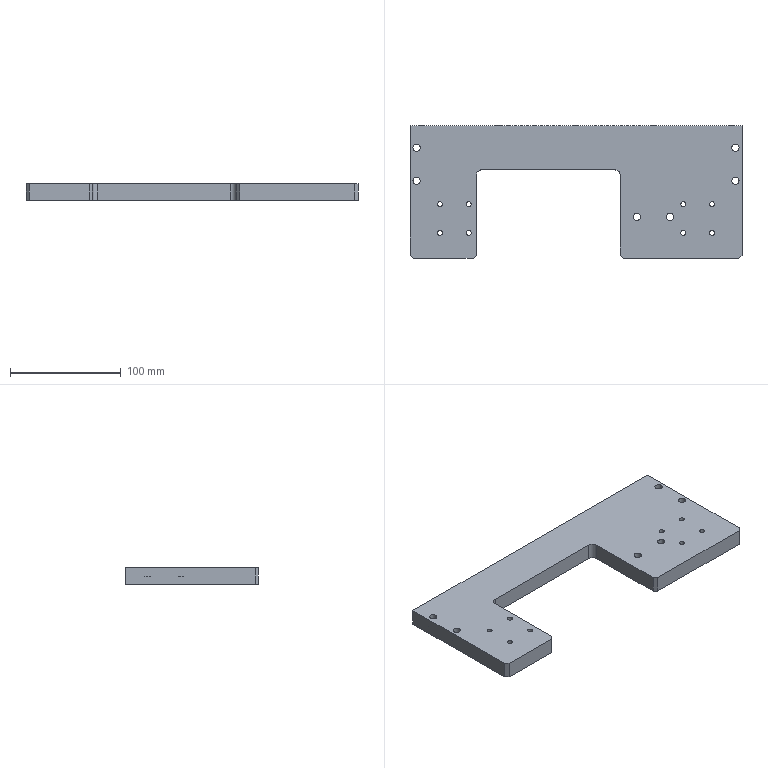Part | NX | 1 solid | 68 faces | box 300 x 120 x 15 mm | volume 373633 mm3 | cylinder 35 | plane 28 | cone 5 | commonest cylinder face diameters 4.5 x8 8 x8 6.6 x6 11 x6 5 x5 10 x2